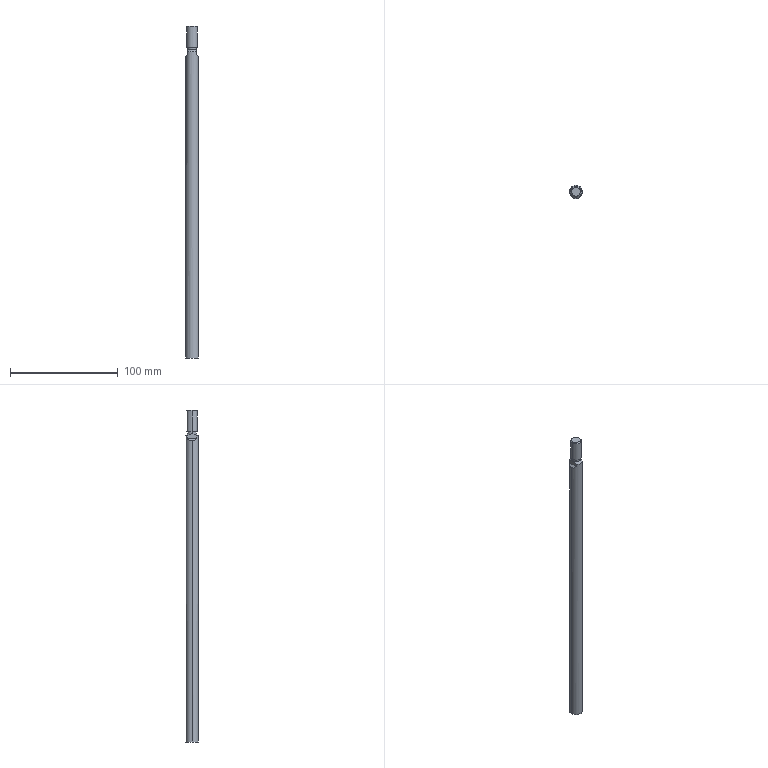Part | STEP file | rod_A_CDM2B32_275_C76_0_ | 1 solid | 19 faces | box 12 x 12 x 308 mm | volume 33830 mm3 | plane 9 | cylinder 6 | cone 4 | commonest cylinder face diameters 8.16 x2 10 x2 12 x2
STEP:
#1=CARTESIAN_POINT('',(6.,0.,-276.));
#2=VERTEX_POINT('',#1);
#3=CARTESIAN_POINT('',(-6.,0.,-276.));
#4=VERTEX_POINT('',#3);
#5=CARTESIAN_POINT('',(0.,0.,-276.));
#6=DIRECTION('',(0.,0.,1.));
#7=DIRECTION('',(1.,0.,0.));
#8=AXIS2_PLACEMENT_3D('',#5,#6,#7);
#9=CIRCLE('',#8,6.);
#10=EDGE_CURVE('',#2,#4,#9,.T.);
#11=ORIENTED_EDGE('',*,*,#10,.T.);
#12=CARTESIAN_POINT('',(-6.,0.,3.5));
#13=VERTEX_POINT('',#12);
#14=CARTESIAN_POINT('',(-6.,0.,-276.));
#15=DIRECTION('',(0.,0.,1.));
#16=VECTOR('',#15,1000.);
#17=LINE('',#14,#16);
#18=EDGE_CURVE('',#4,#13,#17,.T.);
#19=ORIENTED_EDGE('',*,*,#18,.T.);
#20=CARTESIAN_POINT('',(-4.,4.472,5.5));
#21=VERTEX_POINT('',#20);
#22=CARTESIAN_POINT('',(-6.,0.,3.5));
#23=CARTESIAN_POINT('',(-6.,1.734,3.5));
#24=CARTESIAN_POINT('',(-5.292,3.316,4.208));
#25=CARTESIAN_POINT('',(-4.,4.472,5.5));
#26=(BOUNDED_CURVE()B_SPLINE_CURVE(3,(#22,#23,#24,#25),.UNSPECIFIED.,.F.,.F.)B_SPLINE_CURVE_WITH_KNOTS((4,4),(3.142,3.983),.UNSPECIFIED.)CURVE()GEOMETRIC_REPRESENTATION_ITEM()RATIONAL_B_SPLINE_CURVE((1.,0.9419,0.9419,1.))REPRESENTATION_ITEM(''));
#27=EDGE_CURVE('',#13,#21,#26,.T.);
#28=ORIENTED_EDGE('',*,*,#27,.T.);
#29=CARTESIAN_POINT('',(-4.,4.472,8.08));
#30=VERTEX_POINT('',#29);
#31=CARTESIAN_POINT('',(-4.,4.472,-276.));
#32=DIRECTION('',(0.,0.,1.));
#33=VECTOR('',#32,1000.);
#34=LINE('',#31,#33);
#35=EDGE_CURVE('',#21,#30,#34,.T.);
#36=ORIENTED_EDGE('',*,*,#35,.T.);
#37=CARTESIAN_POINT('',(4.,4.472,8.08));
#38=VERTEX_POINT('',#37);
#39=CARTESIAN_POINT('',(0.,0.,8.08));
#40=DIRECTION('',(0.,0.,1.));
#41=DIRECTION('',(1.,0.,0.));
#42=AXIS2_PLACEMENT_3D('',#39,#40,#41);
#43=CIRCLE('',#42,6.);
#44=EDGE_CURVE('',#38,#30,#43,.T.);
#45=ORIENTED_EDGE('',*,*,#44,.F.);
#46=CARTESIAN_POINT('',(4.,4.472,5.5));
#47=VERTEX_POINT('',#46);
#48=CARTESIAN_POINT('',(4.,4.472,-276.));
#49=DIRECTION('',(0.,0.,-1.));
#50=VECTOR('',#49,1000.);
#51=LINE('',#48,#50);
#52=EDGE_CURVE('',#38,#47,#51,.T.);
#53=ORIENTED_EDGE('',*,*,#52,.T.);
#54=CARTESIAN_POINT('',(6.,0.,3.5));
#55=VERTEX_POINT('',#54);
#56=CARTESIAN_POINT('',(4.,4.472,5.5));
#57=CARTESIAN_POINT('',(5.292,3.316,4.208));
#58=CARTESIAN_POINT('',(6.,1.734,3.5));
#59=CARTESIAN_POINT('',(6.,0.,3.5));
#60=(BOUNDED_CURVE()B_SPLINE_CURVE(3,(#56,#57,#58,#59),.UNSPECIFIED.,.F.,.F.)B_SPLINE_CURVE_WITH_KNOTS((4,4),(2.301,3.142),.UNSPECIFIED.)CURVE()GEOMETRIC_REPRESENTATION_ITEM()RATIONAL_B_SPLINE_CURVE((1.,0.9419,0.9419,1.))REPRESENTATION_ITEM(''));
#61=EDGE_CURVE('',#47,#55,#60,.T.);
#62=ORIENTED_EDGE('',*,*,#61,.T.);
#63=CARTESIAN_POINT('',(6.,0.,-276.));
#64=DIRECTION('',(0.,0.,1.));
#65=VECTOR('',#64,1000.);
#66=LINE('',#63,#65);
#67=EDGE_CURVE('',#2,#55,#66,.T.);
#68=ORIENTED_EDGE('',*,*,#67,.F.);
#69=EDGE_LOOP('',(#11,#19,#28,#36,#45,#53,#62,#68));
#70=FACE_OUTER_BOUND('',#69,.T.);
#71=CARTESIAN_POINT('',(0.,0.,-276.));
#72=DIRECTION('',(0.,0.,1.));
#73=DIRECTION('',(1.,0.,0.));
#74=AXIS2_PLACEMENT_3D('',#71,#72,#73);
#75=CYLINDRICAL_SURFACE('',#74,6.);
#76=ADVANCED_FACE('',(#70),#75,.T.);
#77=CARTESIAN_POINT('',(-4.,0.804,10.));
#78=VERTEX_POINT('',#77);
#79=CARTESIAN_POINT('',(-4.08,0.,10.));
#80=VERTEX_POINT('',#79);
#81=CARTESIAN_POINT('',(0.,0.,10.));
#82=DIRECTION('',(0.,0.,1.));
#83=DIRECTION('',(1.,0.,0.));
#84=AXIS2_PLACEMENT_3D('',#81,#82,#83);
#85=CIRCLE('',#84,4.08);
#86=EDGE_CURVE('',#78,#80,#85,.T.);
#87=ORIENTED_EDGE('',*,*,#86,.T.);
#88=CARTESIAN_POINT('',(-4.08,0.,12.5));
#89=VERTEX_POINT('',#88);
#90=CARTESIAN_POINT('',(-4.08,0.,-276.));
#91=DIRECTION('',(0.,0.,1.));
#92=VECTOR('',#91,1000.);
#93=LINE('',#90,#92);
#94=EDGE_CURVE('',#80,#89,#93,.T.);
#95=ORIENTED_EDGE('',*,*,#94,.T.);
#96=CARTESIAN_POINT('',(4.08,0.,12.5));
#97=VERTEX_POINT('',#96);
#98=CARTESIAN_POINT('',(0.,0.,12.5));
#99=DIRECTION('',(0.,0.,1.));
#100=DIRECTION('',(1.,0.,0.));
#101=AXIS2_PLACEMENT_3D('',#98,#99,#100);
#102=CIRCLE('',#101,4.08);
#103=EDGE_CURVE('',#97,#89,#102,.T.);
#104=ORIENTED_EDGE('',*,*,#103,.F.);
#105=CARTESIAN_POINT('',(4.08,0.,10.));
#106=VERTEX_POINT('',#105);
#107=CARTESIAN_POINT('',(4.08,0.,-276.));
#108=DIRECTION('',(0.,0.,1.));
#109=VECTOR('',#108,1000.);
#110=LINE('',#107,#109);
#111=EDGE_CURVE('',#106,#97,#110,.T.);
#112=ORIENTED_EDGE('',*,*,#111,.F.);
#113=CARTESIAN_POINT('',(4.,0.804,10.));
#114=VERTEX_POINT('',#113);
#115=CARTESIAN_POINT('',(0.,0.,10.));
#116=DIRECTION('',(0.,0.,1.));
#117=DIRECTION('',(1.,0.,0.));
#118=AXIS2_PLACEMENT_3D('',#115,#116,#117);
#119=CIRCLE('',#118,4.08);
#120=EDGE_CURVE('',#106,#114,#119,.T.);
#121=ORIENTED_EDGE('',*,*,#120,.T.);
#122=CARTESIAN_POINT('',(0.,0.,10.));
#123=DIRECTION('',(0.,0.,1.));
#124=DIRECTION('',(1.,0.,0.));
#125=AXIS2_PLACEMENT_3D('',#122,#123,#124);
#126=CIRCLE('',#125,4.08);
#127=EDGE_CURVE('',#114,#78,#126,.T.);
#128=ORIENTED_EDGE('',*,*,#127,.T.);
#129=EDGE_LOOP('',(#87,#95,#104,#112,#121,#128));
#130=FACE_OUTER_BOUND('',#129,.T.);
#131=CARTESIAN_POINT('',(0.,0.,-276.));
#132=DIRECTION('',(0.,0.,1.));
#133=DIRECTION('',(1.,0.,0.));
#134=AXIS2_PLACEMENT_3D('',#131,#132,#133);
#135=CYLINDRICAL_SURFACE('',#134,4.08);
#136=ADVANCED_FACE('',(#130),#135,.T.);
#137=CARTESIAN_POINT('',(5.,0.,12.5));
#138=VERTEX_POINT('',#137);
#139=CARTESIAN_POINT('',(-5.,0.,12.5));
#140=VERTEX_POINT('',#139);
#141=CARTESIAN_POINT('',(0.,0.,12.5));
#142=DIRECTION('',(0.,0.,1.));
#143=DIRECTION('',(1.,0.,0.));
#144=AXIS2_PLACEMENT_3D('',#141,#142,#143);
#145=CIRCLE('',#144,5.);
#146=EDGE_CURVE('',#138,#140,#145,.T.);
#147=ORIENTED_EDGE('',*,*,#146,.T.);
#148=CARTESIAN_POINT('',(-5.,0.,31.08));
#149=VERTEX_POINT('',#148);
#150=CARTESIAN_POINT('',(-5.,0.,-276.));
#151=DIRECTION('',(0.,0.,1.));
#152=VECTOR('',#151,1000.);
#153=LINE('',#150,#152);
#154=EDGE_CURVE('',#140,#149,#153,.T.);
#155=ORIENTED_EDGE('',*,*,#154,.T.);
#156=CARTESIAN_POINT('',(5.,0.,31.08));
#157=VERTEX_POINT('',#156);
#158=CARTESIAN_POINT('',(0.,0.,31.08));
#159=DIRECTION('',(0.,0.,1.));
#160=DIRECTION('',(1.,0.,0.));
#161=AXIS2_PLACEMENT_3D('',#158,#159,#160);
#162=CIRCLE('',#161,5.);
#163=EDGE_CURVE('',#157,#149,#162,.T.);
#164=ORIENTED_EDGE('',*,*,#163,.F.);
#165=CARTESIAN_POINT('',(5.,0.,-276.));
#166=DIRECTION('',(0.,0.,1.));
#167=VECTOR('',#166,1000.);
#168=LINE('',#165,#167);
#169=EDGE_CURVE('',#138,#157,#168,.T.);
#170=ORIENTED_EDGE('',*,*,#169,.F.);
#171=EDGE_LOOP('',(#147,#155,#164,#170));
#172=FACE_OUTER_BOUND('',#171,.T.);
#173=CARTESIAN_POINT('',(0.,0.,-276.));
#174=DIRECTION('',(0.,0.,1.));
#175=DIRECTION('',(1.,0.,0.));
#176=AXIS2_PLACEMENT_3D('',#173,#174,#175);
#177=CYLINDRICAL_SURFACE('',#176,5.);
#178=ADVANCED_FACE('',(#172),#177,.T.);
#179=CARTESIAN_POINT('',(4.08,0.,32.));
#180=VERTEX_POINT('',#179);
#181=CARTESIAN_POINT('',(-4.08,0.,32.));
#182=VERTEX_POINT('',#181);
#183=CARTESIAN_POINT('',(0.,0.,32.));
#184=DIRECTION('',(0.,0.,1.));
#185=DIRECTION('',(1.,0.,0.));
#186=AXIS2_PLACEMENT_3D('',#183,#184,#185);
#187=CIRCLE('',#186,4.08);
#188=EDGE_CURVE('',#180,#182,#187,.T.);
#189=ORIENTED_EDGE('',*,*,#188,.F.);
#190=CARTESIAN_POINT('',(5.,0.,31.08));
#191=DIRECTION('',(0.7071,0.,-0.7071));
#192=VECTOR('',#191,1000.);
#193=LINE('',#190,#192);
#194=EDGE_CURVE('',#180,#157,#193,.T.);
#195=ORIENTED_EDGE('',*,*,#194,.T.);
#196=ORIENTED_EDGE('',*,*,#163,.T.);
#197=CARTESIAN_POINT('',(-5.,0.,31.08));
#198=DIRECTION('',(-0.7071,0.,-0.7071));
#199=VECTOR('',#198,1000.);
#200=LINE('',#197,#199);
#201=EDGE_CURVE('',#182,#149,#200,.T.);
#202=ORIENTED_EDGE('',*,*,#201,.F.);
#203=EDGE_LOOP('',(#189,#195,#196,#202));
#204=FACE_OUTER_BOUND('',#203,.T.);
#205=CARTESIAN_POINT('',(0.,0.,31.08));
#206=DIRECTION('',(0.,0.,-1.));
#207=DIRECTION('',(-1.,0.,0.));
#208=AXIS2_PLACEMENT_3D('',#205,#206,#207);
#209=CONICAL_SURFACE('',#208,5.,0.7854);
#210=ADVANCED_FACE('',(#204),#209,.T.);
#211=ORIENTED_EDGE('',*,*,#44,.T.);
#212=CARTESIAN_POINT('',(-4.,4.472,8.08));
#213=CARTESIAN_POINT('',(-4.,4.194,8.287));
#214=CARTESIAN_POINT('',(-4.,3.911,8.49));
#215=CARTESIAN_POINT('',(-4.,3.334,8.877));
#216=CARTESIAN_POINT('',(-4.,3.038,9.063));
#217=CARTESIAN_POINT('',(-4.,2.432,9.405));
#218=CARTESIAN_POINT('',(-4.,2.122,9.561));
#219=CARTESIAN_POINT('',(-4.,1.478,9.826));
#220=CARTESIAN_POINT('',(-4.,1.143,9.933));
#221=CARTESIAN_POINT('',(-4.,0.804,10.));
#222=B_SPLINE_CURVE_WITH_KNOTS('',3,(#212,#213,#214,#215,#216,#217,#218,#219,#220,#221),.UNSPECIFIED.,.F.,.F.,(4,2,2,2,4),(0.01098,0.01203,0.01307,0.01411,0.01515),.UNSPECIFIED.);
#223=EDGE_CURVE('',#30,#78,#222,.T.);
#224=ORIENTED_EDGE('',*,*,#223,.T.);
#225=ORIENTED_EDGE('',*,*,#127,.F.);
#226=CARTESIAN_POINT('',(4.,0.804,10.));
#227=CARTESIAN_POINT('',(4.,1.145,9.933));
#228=CARTESIAN_POINT('',(4.,1.483,9.824));
#229=CARTESIAN_POINT('',(4.,2.128,9.559));
#230=CARTESIAN_POINT('',(4.,2.437,9.403));
#231=CARTESIAN_POINT('',(4.,3.341,8.892));
#232=CARTESIAN_POINT('',(4.,3.914,8.496));
#233=CARTESIAN_POINT('',(4.,4.472,8.08));
#234=B_SPLINE_CURVE_WITH_KNOTS('',3,(#226,#227,#228,#229,#230,#231,#232,#233),.UNSPECIFIED.,.F.,.F.,(4,2,2,4),(0.01677,0.01782,0.01887,0.02097),.UNSPECIFIED.);
#235=EDGE_CURVE('',#114,#38,#234,.T.);
#236=ORIENTED_EDGE('',*,*,#235,.T.);
#237=EDGE_LOOP('',(#211,#224,#225,#236));
#238=FACE_OUTER_BOUND('',#237,.T.);
#239=CARTESIAN_POINT('',(0.,0.,8.08));
#240=DIRECTION('',(0.,0.,-1.));
#241=DIRECTION('',(-1.,0.,0.));
#242=AXIS2_PLACEMENT_3D('',#239,#240,#241);
#243=CONICAL_SURFACE('',#242,6.,0.7854);
#244=ADVANCED_FACE('',(#238),#243,.T.);
#245=CARTESIAN_POINT('',(0.,0.,32.));
#246=DIRECTION('',(0.,0.,1.));
#247=DIRECTION('',(1.,0.,0.));
#248=AXIS2_PLACEMENT_3D('',#245,#246,#247);
#249=CIRCLE('',#248,4.08);
#250=EDGE_CURVE('',#182,#180,#249,.T.);
#251=ORIENTED_EDGE('',*,*,#250,.T.);
#252=ORIENTED_EDGE('',*,*,#188,.T.);
#253=EDGE_LOOP('',(#251,#252));
#254=FACE_OUTER_BOUND('',#253,.T.);
#255=CARTESIAN_POINT('',(0.,0.,32.));
#256=DIRECTION('',(0.,0.,-1.));
#257=DIRECTION('',(-1.,0.,0.));
#258=AXIS2_PLACEMENT_3D('',#255,#256,#257);
#259=PLANE('',#258);
#260=ADVANCED_FACE('',(#254),#259,.F.);
#261=ORIENTED_EDGE('',*,*,#194,.F.);
#262=ORIENTED_EDGE('',*,*,#250,.F.);
#263=ORIENTED_EDGE('',*,*,#201,.T.);
#264=CARTESIAN_POINT('',(0.,0.,31.08));
#265=DIRECTION('',(0.,0.,1.));
#266=DIRECTION('',(1.,0.,0.));
#267=AXIS2_PLACEMENT_3D('',#264,#265,#266);
#268=CIRCLE('',#267,5.);
#269=EDGE_CURVE('',#149,#157,#268,.T.);
#270=ORIENTED_EDGE('',*,*,#269,.T.);
#271=EDGE_LOOP('',(#261,#262,#263,#270));
#272=FACE_OUTER_BOUND('',#271,.T.);
#273=CARTESIAN_POINT('',(0.,0.,31.08));
#274=DIRECTION('',(0.,0.,-1.));
#275=DIRECTION('',(-1.,0.,0.));
#276=AXIS2_PLACEMENT_3D('',#273,#274,#275);
#277=CONICAL_SURFACE('',#276,5.,0.7854);
#278=ADVANCED_FACE('',(#272),#277,.T.);
#279=ORIENTED_EDGE('',*,*,#154,.F.);
#280=CARTESIAN_POINT('',(0.,0.,12.5));
#281=DIRECTION('',(0.,0.,1.));
#282=DIRECTION('',(1.,0.,0.));
#283=AXIS2_PLACEMENT_3D('',#280,#281,#282);
#284=CIRCLE('',#283,5.);
#285=EDGE_CURVE('',#140,#138,#284,.T.);
#286=ORIENTED_EDGE('',*,*,#285,.T.);
#287=ORIENTED_EDGE('',*,*,#169,.T.);
#288=ORIENTED_EDGE('',*,*,#269,.F.);
#289=EDGE_LOOP('',(#279,#286,#287,#288));
#290=FACE_OUTER_BOUND('',#289,.T.);
#291=CARTESIAN_POINT('',(0.,0.,-276.));
#292=DIRECTION('',(0.,0.,1.));
#293=DIRECTION('',(1.,0.,0.));
#294=AXIS2_PLACEMENT_3D('',#291,#292,#293);
#295=CYLINDRICAL_SURFACE('',#294,5.);
#296=ADVANCED_FACE('',(#290),#295,.T.);
#297=ORIENTED_EDGE('',*,*,#146,.F.);
#298=ORIENTED_EDGE('',*,*,#285,.F.);
#299=EDGE_LOOP('',(#297,#298));
#300=FACE_OUTER_BOUND('',#299,.T.);
#301=ORIENTED_EDGE('',*,*,#103,.T.);
#302=CARTESIAN_POINT('',(0.,0.,12.5));
#303=DIRECTION('',(0.,0.,1.));
#304=DIRECTION('',(1.,0.,0.));
#305=AXIS2_PLACEMENT_3D('',#302,#303,#304);
#306=CIRCLE('',#305,4.08);
#307=EDGE_CURVE('',#89,#97,#306,.T.);
#308=ORIENTED_EDGE('',*,*,#307,.T.);
#309=EDGE_LOOP('',(#301,#308));
#310=FACE_BOUND('',#309,.T.);
#311=CARTESIAN_POINT('',(0.,5.,12.5));
#312=DIRECTION('',(0.,0.,1.));
#313=DIRECTION('',(1.,0.,0.));
#314=AXIS2_PLACEMENT_3D('',#311,#312,#313);
#315=PLANE('',#314);
#316=ADVANCED_FACE('',(#300,#310),#315,.F.);
#317=ORIENTED_EDGE('',*,*,#94,.F.);
#318=CARTESIAN_POINT('',(-4.,-0.804,10.));
#319=VERTEX_POINT('',#318);
#320=CARTESIAN_POINT('',(0.,0.,10.));
#321=DIRECTION('',(0.,0.,1.));
#322=DIRECTION('',(1.,0.,0.));
#323=AXIS2_PLACEMENT_3D('',#320,#321,#322);
#324=CIRCLE('',#323,4.08);
#325=EDGE_CURVE('',#80,#319,#324,.T.);
#326=ORIENTED_EDGE('',*,*,#325,.T.);
#327=CARTESIAN_POINT('',(4.,-0.804,10.));
#328=VERTEX_POINT('',#327);
#329=CARTESIAN_POINT('',(0.,0.,10.));
#330=DIRECTION('',(0.,0.,1.));
#331=DIRECTION('',(1.,0.,0.));
#332=AXIS2_PLACEMENT_3D('',#329,#330,#331);
#333=CIRCLE('',#332,4.08);
#334=EDGE_CURVE('',#319,#328,#333,.T.);
#335=ORIENTED_EDGE('',*,*,#334,.T.);
#336=CARTESIAN_POINT('',(0.,0.,10.));
#337=DIRECTION('',(0.,0.,1.));
#338=DIRECTION('',(1.,0.,0.));
#339=AXIS2_PLACEMENT_3D('',#336,#337,#338);
#340=CIRCLE('',#339,4.08);
#341=EDGE_CURVE('',#328,#106,#340,.T.);
#342=ORIENTED_EDGE('',*,*,#341,.T.);
#343=ORIENTED_EDGE('',*,*,#111,.T.);
#344=ORIENTED_EDGE('',*,*,#307,.F.);
#345=EDGE_LOOP('',(#317,#326,#335,#342,#343,#344));
#346=FACE_OUTER_BOUND('',#345,.T.);
#347=CARTESIAN_POINT('',(0.,0.,-276.));
#348=DIRECTION('',(0.,0.,1.));
#349=DIRECTION('',(1.,0.,0.));
#350=AXIS2_PLACEMENT_3D('',#347,#348,#349);
#351=CYLINDRICAL_SURFACE('',#350,4.08);
#352=ADVANCED_FACE('',(#346),#351,.T.);
#353=ORIENTED_EDGE('',*,*,#334,.F.);
#354=CARTESIAN_POINT('',(-4.,-4.472,8.08));
#355=VERTEX_POINT('',#354);
#356=CARTESIAN_POINT('',(-4.,-0.804,10.));
#357=CARTESIAN_POINT('',(-4.,-1.145,9.933));
#358=CARTESIAN_POINT('',(-4.,-1.483,9.824));
#359=CARTESIAN_POINT('',(-4.,-2.128,9.559));
#360=CARTESIAN_POINT('',(-4.,-2.437,9.403));
#361=CARTESIAN_POINT('',(-4.,-3.341,8.892));
#362=CARTESIAN_POINT('',(-4.,-3.914,8.496));
#363=CARTESIAN_POINT('',(-4.,-4.472,8.08));
#364=B_SPLINE_CURVE_WITH_KNOTS('',3,(#356,#357,#358,#359,#360,#361,#362,#363),.UNSPECIFIED.,.F.,.F.,(4,2,2,4),(0.01677,0.01782,0.01887,0.02097),.UNSPECIFIED.);
#365=EDGE_CURVE('',#319,#355,#364,.T.);
#366=ORIENTED_EDGE('',*,*,#365,.T.);
#367=CARTESIAN_POINT('',(4.,-4.472,8.08));
#368=VERTEX_POINT('',#367);
#369=CARTESIAN_POINT('',(0.,0.,8.08));
#370=DIRECTION('',(0.,0.,1.));
#371=DIRECTION('',(1.,0.,0.));
#372=AXIS2_PLACEMENT_3D('',#369,#370,#371);
#373=CIRCLE('',#372,6.);
#374=EDGE_CURVE('',#355,#368,#373,.T.);
#375=ORIENTED_EDGE('',*,*,#374,.T.);
#376=CARTESIAN_POINT('',(4.,-4.472,8.08));
#377=CARTESIAN_POINT('',(4.,-4.194,8.287));
#378=CARTESIAN_POINT('',(4.,-3.911,8.49));
#379=CARTESIAN_POINT('',(4.,-3.334,8.877));
#380=CARTESIAN_POINT('',(4.,-3.038,9.063));
#381=CARTESIAN_POINT('',(4.,-2.432,9.405));
#382=CARTESIAN_POINT('',(4.,-2.122,9.561));
#383=CARTESIAN_POINT('',(4.,-1.478,9.826));
#384=CARTESIAN_POINT('',(4.,-1.143,9.933));
#385=CARTESIAN_POINT('',(4.,-0.804,10.));
#386=B_SPLINE_CURVE_WITH_KNOTS('',3,(#376,#377,#378,#379,#380,#381,#382,#383,#384,#385),.UNSPECIFIED.,.F.,.F.,(4,2,2,2,4),(0.01098,0.01203,0.01307,0.01411,0.01515),.UNSPECIFIED.);
#387=EDGE_CURVE('',#368,#328,#386,.T.);
#388=ORIENTED_EDGE('',*,*,#387,.T.);
#389=EDGE_LOOP('',(#353,#366,#375,#388));
#390=FACE_OUTER_BOUND('',#389,.T.);
#391=CARTESIAN_POINT('',(0.,0.,8.08));
#392=DIRECTION('',(0.,0.,-1.));
#393=DIRECTION('',(-1.,0.,0.));
#394=AXIS2_PLACEMENT_3D('',#391,#392,#393);
#395=CONICAL_SURFACE('',#394,6.,0.7854);
#396=ADVANCED_FACE('',(#390),#395,.T.);
#397=ORIENTED_EDGE('',*,*,#18,.F.);
#398=CARTESIAN_POINT('',(0.,0.,-276.));
#399=DIRECTION('',(0.,0.,1.));
#400=DIRECTION('',(1.,0.,0.));
#401=AXIS2_PLACEMENT_3D('',#398,#399,#400);
#402=CIRCLE('',#401,6.);
#403=EDGE_CURVE('',#4,#2,#402,.T.);
#404=ORIENTED_EDGE('',*,*,#403,.T.);
#405=ORIENTED_EDGE('',*,*,#67,.T.);
#406=CARTESIAN_POINT('',(4.,-4.472,5.5));
#407=VERTEX_POINT('',#406);
#408=CARTESIAN_POINT('',(6.,0.,3.5));
#409=CARTESIAN_POINT('',(6.,-1.734,3.5));
#410=CARTESIAN_POINT('',(5.292,-3.316,4.208));
#411=CARTESIAN_POINT('',(4.,-4.472,5.5));
#412=(BOUNDED_CURVE()B_SPLINE_CURVE(3,(#408,#409,#410,#411),.UNSPECIFIED.,.F.,.T.)B_SPLINE_CURVE_WITH_KNOTS((4,4),(3.142,3.983),.UNSPECIFIED.)CURVE()GEOMETRIC_REPRESENTATION_ITEM()RATIONAL_B_SPLINE_CURVE((1.,0.9419,0.9419,1.))REPRESENTATION_ITEM(''));
#413=EDGE_CURVE('',#55,#407,#412,.T.);
#414=ORIENTED_EDGE('',*,*,#413,.T.);
#415=CARTESIAN_POINT('',(4.,-4.472,-276.));
#416=DIRECTION('',(0.,0.,1.));
#417=VECTOR('',#416,1000.);
#418=LINE('',#415,#417);
#419=EDGE_CURVE('',#407,#368,#418,.T.);
#420=ORIENTED_EDGE('',*,*,#419,.T.);
#421=ORIENTED_EDGE('',*,*,#374,.F.);
#422=CARTESIAN_POINT('',(-4.,-4.472,5.5));
#423=VERTEX_POINT('',#422);
#424=CARTESIAN_POINT('',(-4.,-4.472,-276.));
#425=DIRECTION('',(0.,0.,-1.));
#426=VECTOR('',#425,1000.);
#427=LINE('',#424,#426);
#428=EDGE_CURVE('',#355,#423,#427,.T.);
#429=ORIENTED_EDGE('',*,*,#428,.T.);
#430=CARTESIAN_POINT('',(-4.,-4.472,5.5));
#431=CARTESIAN_POINT('',(-5.292,-3.316,4.208));
#432=CARTESIAN_POINT('',(-6.,-1.734,3.5));
#433=CARTESIAN_POINT('',(-6.,0.,3.5));
#434=(BOUNDED_CURVE()B_SPLINE_CURVE(3,(#430,#431,#432,#433),.UNSPECIFIED.,.F.,.F.)B_SPLINE_CURVE_WITH_KNOTS((4,4),(2.301,3.142),.UNSPECIFIED.)CURVE()GEOMETRIC_REPRESENTATION_ITEM()RATIONAL_B_SPLINE_CURVE((1.,0.9419,0.9419,1.))REPRESENTATION_ITEM(''));
#435=EDGE_CURVE('',#423,#13,#434,.T.);
#436=ORIENTED_EDGE('',*,*,#435,.T.);
#437=EDGE_LOOP('',(#397,#404,#405,#414,#420,#421,#429,#436));
#438=FACE_OUTER_BOUND('',#437,.T.);
#439=CARTESIAN_POINT('',(0.,0.,-276.));
#440=DIRECTION('',(0.,0.,1.));
#441=DIRECTION('',(1.,0.,0.));
#442=AXIS2_PLACEMENT_3D('',#439,#440,#441);
#443=CYLINDRICAL_SURFACE('',#442,6.);
#444=ADVANCED_FACE('',(#438),#443,.T.);
#445=ORIENTED_EDGE('',*,*,#10,.F.);
#446=ORIENTED_EDGE('',*,*,#403,.F.);
#447=EDGE_LOOP('',(#445,#446));
#448=FACE_OUTER_BOUND('',#447,.T.);
#449=CARTESIAN_POINT('',(0.,6.,-276.));
#450=DIRECTION('',(0.,0.,1.));
#451=DIRECTION('',(1.,0.,0.));
#452=AXIS2_PLACEMENT_3D('',#449,#450,#451);
#453=PLANE('',#452);
#454=ADVANCED_FACE('',(#448),#453,.F.);
#455=CARTESIAN_POINT('',(4.,-12.,10.));
#456=DIRECTION('',(0.,1.,0.));
#457=VECTOR('',#456,1000.);
#458=LINE('',#455,#457);
#459=EDGE_CURVE('',#328,#114,#458,.T.);
#460=ORIENTED_EDGE('',*,*,#459,.T.);
#461=ORIENTED_EDGE('',*,*,#120,.F.);
#462=ORIENTED_EDGE('',*,*,#341,.F.);
#463=EDGE_LOOP('',(#460,#461,#462));
#464=FACE_OUTER_BOUND('',#463,.T.);
#465=CARTESIAN_POINT('',(4.,-12.,10.));
#466=DIRECTION('',(0.,0.,1.));
#467=DIRECTION('',(1.,0.,0.));
#468=AXIS2_PLACEMENT_3D('',#465,#466,#467);
#469=PLANE('',#468);
#470=ADVANCED_FACE('',(#464),#469,.F.);
#471=ORIENTED_EDGE('',*,*,#419,.F.);
#472=CARTESIAN_POINT('',(4.,-12.,5.5));
#473=DIRECTION('',(0.,1.,0.));
#474=VECTOR('',#473,1000.);
#475=LINE('',#472,#474);
#476=EDGE_CURVE('',#407,#47,#475,.T.);
#477=ORIENTED_EDGE('',*,*,#476,.T.);
#478=ORIENTED_EDGE('',*,*,#52,.F.);
#479=ORIENTED_EDGE('',*,*,#235,.F.);
#480=ORIENTED_EDGE('',*,*,#459,.F.);
#481=ORIENTED_EDGE('',*,*,#387,.F.);
#482=EDGE_LOOP('',(#471,#477,#478,#479,#480,#481));
#483=FACE_OUTER_BOUND('',#482,.T.);
#484=CARTESIAN_POINT('',(4.,-12.,5.5));
#485=DIRECTION('',(-1.,0.,0.));
#486=DIRECTION('',(0.,0.,1.));
#487=AXIS2_PLACEMENT_3D('',#484,#485,#486);
#488=PLANE('',#487);
#489=ADVANCED_FACE('',(#483),#488,.F.);
#490=ORIENTED_EDGE('',*,*,#476,.F.);
#491=ORIENTED_EDGE('',*,*,#413,.F.);
#492=ORIENTED_EDGE('',*,*,#61,.F.);
#493=EDGE_LOOP('',(#490,#491,#492));
#494=FACE_OUTER_BOUND('',#493,.T.);
#495=CARTESIAN_POINT('',(6.,-12.,3.5));
#496=DIRECTION('',(-0.7071,0.,-0.7071));
#497=DIRECTION('',(-0.7071,0.,0.7071));
#498=AXIS2_PLACEMENT_3D('',#495,#496,#497);
#499=PLANE('',#498);
#500=ADVANCED_FACE('',(#494),#499,.F.);
#501=CARTESIAN_POINT('',(-4.,-12.,10.));
#502=DIRECTION('',(0.,1.,0.));
#503=VECTOR('',#502,1000.);
#504=LINE('',#501,#503);
#505=EDGE_CURVE('',#319,#78,#504,.T.);
#506=ORIENTED_EDGE('',*,*,#505,.F.);
#507=ORIENTED_EDGE('',*,*,#325,.F.);
#508=ORIENTED_EDGE('',*,*,#86,.F.);
#509=EDGE_LOOP('',(#506,#507,#508));
#510=FACE_OUTER_BOUND('',#509,.T.);
#511=CARTESIAN_POINT('',(-8.,-12.,10.));
#512=DIRECTION('',(0.,0.,1.));
#513=DIRECTION('',(1.,0.,0.));
#514=AXIS2_PLACEMENT_3D('',#511,#512,#513);
#515=PLANE('',#514);
#516=ADVANCED_FACE('',(#510),#515,.F.);
#517=CARTESIAN_POINT('',(-4.,-12.,5.5));
#518=DIRECTION('',(0.,1.,0.));
#519=VECTOR('',#518,1000.);
#520=LINE('',#517,#519);
#521=EDGE_CURVE('',#423,#21,#520,.T.);
#522=ORIENTED_EDGE('',*,*,#521,.T.);
#523=ORIENTED_EDGE('',*,*,#27,.F.);
#524=ORIENTED_EDGE('',*,*,#435,.F.);
#525=EDGE_LOOP('',(#522,#523,#524));
#526=FACE_OUTER_BOUND('',#525,.T.);
#527=CARTESIAN_POINT('',(-4.,-12.,5.5));
#528=DIRECTION('',(0.7071,0.,-0.7071));
#529=DIRECTION('',(-0.7071,0.,-0.7071));
#530=AXIS2_PLACEMENT_3D('',#527,#528,#529);
#531=PLANE('',#530);
#532=ADVANCED_FACE('',(#526),#531,.F.);
#533=ORIENTED_EDGE('',*,*,#35,.F.);
#534=ORIENTED_EDGE('',*,*,#521,.F.);
#535=ORIENTED_EDGE('',*,*,#428,.F.);
#536=ORIENTED_EDGE('',*,*,#365,.F.);
#537=ORIENTED_EDGE('',*,*,#505,.T.);
#538=ORIENTED_EDGE('',*,*,#223,.F.);
#539=EDGE_LOOP('',(#533,#534,#535,#536,#537,#538));
#540=FACE_OUTER_BOUND('',#539,.T.);
#541=CARTESIAN_POINT('',(-4.,-12.,10.));
#542=DIRECTION('',(1.,0.,0.));
#543=DIRECTION('',(0.,0.,-1.));
#544=AXIS2_PLACEMENT_3D('',#541,#542,#543);
#545=PLANE('',#544);
#546=ADVANCED_FACE('',(#540),#545,.F.);
#547=CLOSED_SHELL('',(#76,#136,#178,#210,#244,#260,#278,#296,#316,#352,#396,#444,#454,#470,#489,#500,#516,#532,#546));
#548=MANIFOLD_SOLID_BREP('',#547);
#549=CARTESIAN_POINT('',(0.,0.,0.));
#550=DIRECTION('',(0.,0.,1.));
#551=DIRECTION('',(1.,0.,0.));
#552=AXIS2_PLACEMENT_3D('',#549,#550,#551);
#553=(LENGTH_UNIT()NAMED_UNIT(*)SI_UNIT(.MILLI.,.METRE.));
#554=UNCERTAINTY_MEASURE_WITH_UNIT(LENGTH_MEASURE(0.00001),#553,'','');
#555=(NAMED_UNIT(*)PLANE_ANGLE_UNIT()SI_UNIT($,.RADIAN.));
#556=(NAMED_UNIT(*)SI_UNIT($,.STERADIAN.)SOLID_ANGLE_UNIT());
#557=(GEOMETRIC_REPRESENTATION_CONTEXT(3)GLOBAL_UNCERTAINTY_ASSIGNED_CONTEXT((#554))GLOBAL_UNIT_ASSIGNED_CONTEXT((#553,#555,#556))REPRESENTATION_CONTEXT('',''));
#558=ADVANCED_BREP_SHAPE_REPRESENTATION('',(#548,#552),#557);